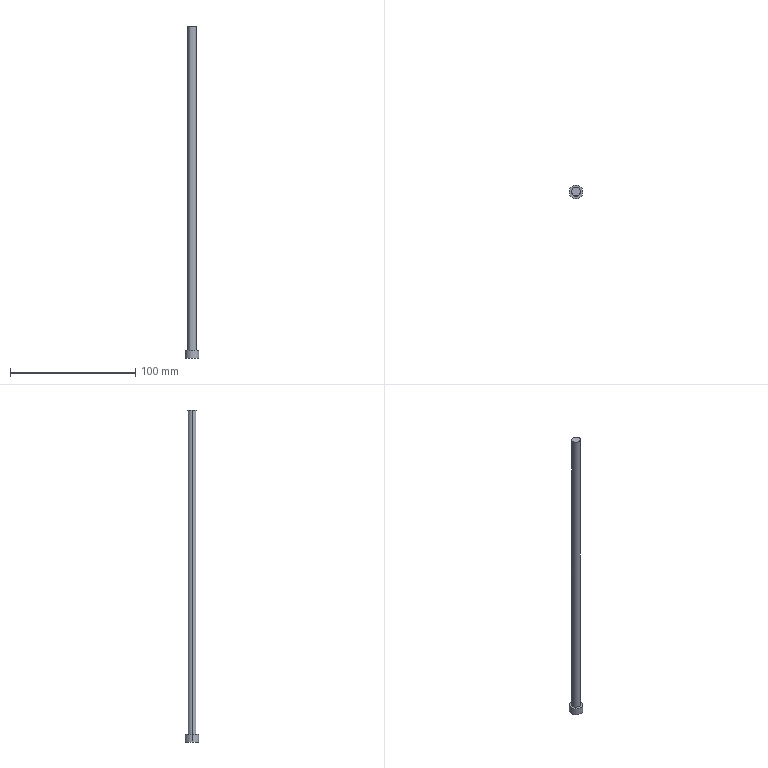Part | Creo | 1 solid | 7 faces | box 11 x 11 x 265.581 mm | volume 10560 mm3 | cylinder 4 | plane 3 | commonest cylinder face diameters 7 x2 11 x2
STEP:
#1=CARTESIAN_POINT('',(0.,0.,0.));
#2=DIRECTION('',(0.,0.,1.));
#3=DIRECTION('',(1.,0.,0.));
#4=AXIS2_PLACEMENT_3D('',#1,#2,#3);
#5=CARTESIAN_POINT('',(3.5,-45.2,-219.5));
#6=VERTEX_POINT('',#5);
#7=CARTESIAN_POINT('',(10.5,-45.2,-219.5));
#8=VERTEX_POINT('',#7);
#9=CARTESIAN_POINT('',(7.,-45.2,-219.5));
#10=DIRECTION('',(0.,0.,-1.));
#11=DIRECTION('',(-1.,0.,0.));
#12=AXIS2_PLACEMENT_3D('',#9,#10,#11);
#13=CIRCLE('',#12,3.5);
#14=EDGE_CURVE('',#6,#8,#13,.T.);
#15=ORIENTED_EDGE('',*,*,#14,.T.);
#16=CARTESIAN_POINT('',(10.5,-45.2,40.081));
#17=VERTEX_POINT('',#16);
#18=CARTESIAN_POINT('',(10.5,-45.2,40.081));
#19=DIRECTION('',(0.,0.,-1.));
#20=VECTOR('',#19,259.581);
#21=LINE('',#18,#20);
#22=EDGE_CURVE('',#17,#8,#21,.T.);
#23=ORIENTED_EDGE('',*,*,#22,.F.);
#24=CARTESIAN_POINT('',(3.5,-45.2,40.081));
#25=VERTEX_POINT('',#24);
#26=CARTESIAN_POINT('',(7.,-45.2,40.081));
#27=DIRECTION('',(0.,0.,1.));
#28=DIRECTION('',(1.,0.,0.));
#29=AXIS2_PLACEMENT_3D('',#26,#27,#28);
#30=CIRCLE('',#29,3.5);
#31=EDGE_CURVE('',#17,#25,#30,.T.);
#32=ORIENTED_EDGE('',*,*,#31,.T.);
#33=CARTESIAN_POINT('',(3.5,-45.2,40.081));
#34=DIRECTION('',(0.,0.,-1.));
#35=VECTOR('',#34,259.581);
#36=LINE('',#33,#35);
#37=EDGE_CURVE('',#25,#6,#36,.T.);
#38=ORIENTED_EDGE('',*,*,#37,.T.);
#39=EDGE_LOOP('',(#15,#23,#32,#38));
#40=FACE_OUTER_BOUND('',#39,.F.);
#41=CARTESIAN_POINT('',(7.,-45.2,125.91));
#42=DIRECTION('',(0.,0.,-1.));
#43=DIRECTION('',(-1.,0.,0.));
#44=AXIS2_PLACEMENT_3D('',#41,#42,#43);
#45=CYLINDRICAL_SURFACE('',#44,3.5);
#46=ADVANCED_FACE('',(#40),#45,.T.);
#47=CARTESIAN_POINT('',(1.5,-45.2,-219.5));
#48=VERTEX_POINT('',#47);
#49=CARTESIAN_POINT('',(12.5,-45.2,-219.5));
#50=VERTEX_POINT('',#49);
#51=CARTESIAN_POINT('',(7.,-45.2,-219.5));
#52=DIRECTION('',(0.,0.,1.));
#53=DIRECTION('',(-1.,0.,0.));
#54=AXIS2_PLACEMENT_3D('',#51,#52,#53);
#55=CIRCLE('',#54,5.5);
#56=EDGE_CURVE('',#48,#50,#55,.T.);
#57=ORIENTED_EDGE('',*,*,#56,.F.);
#58=CARTESIAN_POINT('',(7.,-45.2,-219.5));
#59=DIRECTION('',(0.,0.,1.));
#60=DIRECTION('',(1.,0.,0.));
#61=AXIS2_PLACEMENT_3D('',#58,#59,#60);
#62=CIRCLE('',#61,5.5);
#63=EDGE_CURVE('',#50,#48,#62,.T.);
#64=ORIENTED_EDGE('',*,*,#63,.F.);
#65=EDGE_LOOP('',(#57,#64));
#66=FACE_OUTER_BOUND('',#65,.F.);
#67=ORIENTED_EDGE('',*,*,#14,.F.);
#68=CARTESIAN_POINT('',(7.,-45.2,-219.5));
#69=DIRECTION('',(0.,0.,-1.));
#70=DIRECTION('',(1.,0.,0.));
#71=AXIS2_PLACEMENT_3D('',#68,#69,#70);
#72=CIRCLE('',#71,3.5);
#73=EDGE_CURVE('',#8,#6,#72,.T.);
#74=ORIENTED_EDGE('',*,*,#73,.F.);
#75=EDGE_LOOP('',(#67,#74));
#76=FACE_BOUND('',#75,.F.);
#77=CARTESIAN_POINT('',(-30.,-4.2,-219.5));
#78=DIRECTION('',(0.,0.,-1.));
#79=DIRECTION('',(-1.,0.,0.));
#80=AXIS2_PLACEMENT_3D('',#77,#78,#79);
#81=PLANE('',#80);
#82=ADVANCED_FACE('',(#66,#76),#81,.F.);
#83=CARTESIAN_POINT('',(12.5,-45.2,-225.5));
#84=VERTEX_POINT('',#83);
#85=CARTESIAN_POINT('',(1.5,-45.2,-225.5));
#86=VERTEX_POINT('',#85);
#87=CARTESIAN_POINT('',(7.,-45.2,-225.5));
#88=DIRECTION('',(0.,0.,-1.));
#89=DIRECTION('',(1.,0.,0.));
#90=AXIS2_PLACEMENT_3D('',#87,#88,#89);
#91=CIRCLE('',#90,5.5);
#92=EDGE_CURVE('',#84,#86,#91,.T.);
#93=ORIENTED_EDGE('',*,*,#92,.T.);
#94=CARTESIAN_POINT('',(1.5,-45.2,-225.5));
#95=DIRECTION('',(0.,0.,1.));
#96=VECTOR('',#95,6.);
#97=LINE('',#94,#96);
#98=EDGE_CURVE('',#86,#48,#97,.T.);
#99=ORIENTED_EDGE('',*,*,#98,.T.);
#100=ORIENTED_EDGE('',*,*,#56,.T.);
#101=CARTESIAN_POINT('',(12.5,-45.2,-225.5));
#102=DIRECTION('',(0.,0.,1.));
#103=VECTOR('',#102,6.);
#104=LINE('',#101,#103);
#105=EDGE_CURVE('',#84,#50,#104,.T.);
#106=ORIENTED_EDGE('',*,*,#105,.F.);
#107=EDGE_LOOP('',(#93,#99,#100,#106));
#108=FACE_OUTER_BOUND('',#107,.F.);
#109=CARTESIAN_POINT('',(7.,-45.2,-225.5));
#110=DIRECTION('',(0.,0.,1.));
#111=DIRECTION('',(1.,0.,0.));
#112=AXIS2_PLACEMENT_3D('',#109,#110,#111);
#113=CYLINDRICAL_SURFACE('',#112,5.5);
#114=ADVANCED_FACE('',(#108),#113,.T.);
#115=CARTESIAN_POINT('',(7.,-45.2,-225.5));
#116=DIRECTION('',(0.,0.,-1.));
#117=DIRECTION('',(-1.,0.,0.));
#118=AXIS2_PLACEMENT_3D('',#115,#116,#117);
#119=CIRCLE('',#118,5.5);
#120=EDGE_CURVE('',#86,#84,#119,.T.);
#121=ORIENTED_EDGE('',*,*,#120,.F.);
#122=ORIENTED_EDGE('',*,*,#92,.F.);
#123=EDGE_LOOP('',(#121,#122));
#124=FACE_OUTER_BOUND('',#123,.F.);
#125=CARTESIAN_POINT('',(-30.,-4.2,-225.5));
#126=DIRECTION('',(0.,0.,-1.));
#127=DIRECTION('',(-1.,0.,0.));
#128=AXIS2_PLACEMENT_3D('',#125,#126,#127);
#129=PLANE('',#128);
#130=ADVANCED_FACE('',(#124),#129,.T.);
#131=ORIENTED_EDGE('',*,*,#120,.T.);
#132=ORIENTED_EDGE('',*,*,#105,.T.);
#133=ORIENTED_EDGE('',*,*,#63,.T.);
#134=ORIENTED_EDGE('',*,*,#98,.F.);
#135=EDGE_LOOP('',(#131,#132,#133,#134));
#136=FACE_OUTER_BOUND('',#135,.F.);
#137=CARTESIAN_POINT('',(7.,-45.2,-225.5));
#138=DIRECTION('',(0.,0.,1.));
#139=DIRECTION('',(1.,0.,0.));
#140=AXIS2_PLACEMENT_3D('',#137,#138,#139);
#141=CYLINDRICAL_SURFACE('',#140,5.5);
#142=ADVANCED_FACE('',(#136),#141,.T.);
#143=ORIENTED_EDGE('',*,*,#73,.T.);
#144=ORIENTED_EDGE('',*,*,#37,.F.);
#145=CARTESIAN_POINT('',(7.,-45.2,40.081));
#146=DIRECTION('',(0.,0.,1.));
#147=DIRECTION('',(-1.,0.,0.));
#148=AXIS2_PLACEMENT_3D('',#145,#146,#147);
#149=CIRCLE('',#148,3.5);
#150=EDGE_CURVE('',#25,#17,#149,.T.);
#151=ORIENTED_EDGE('',*,*,#150,.T.);
#152=ORIENTED_EDGE('',*,*,#22,.T.);
#153=EDGE_LOOP('',(#143,#144,#151,#152));
#154=FACE_OUTER_BOUND('',#153,.F.);
#155=CARTESIAN_POINT('',(7.,-45.2,125.91));
#156=DIRECTION('',(0.,0.,-1.));
#157=DIRECTION('',(-1.,0.,0.));
#158=AXIS2_PLACEMENT_3D('',#155,#156,#157);
#159=CYLINDRICAL_SURFACE('',#158,3.5);
#160=ADVANCED_FACE('',(#154),#159,.T.);
#161=ORIENTED_EDGE('',*,*,#31,.F.);
#162=ORIENTED_EDGE('',*,*,#150,.F.);
#163=EDGE_LOOP('',(#161,#162));
#164=FACE_OUTER_BOUND('',#163,.F.);
#165=CARTESIAN_POINT('',(-11.653,-0.6637,40.081));
#166=DIRECTION('',(0.,0.,1.));
#167=DIRECTION('',(1.,0.,0.));
#168=AXIS2_PLACEMENT_3D('',#165,#166,#167);
#169=PLANE('',#168);
#170=ADVANCED_FACE('',(#164),#169,.T.);
#171=CLOSED_SHELL('',(#46,#82,#114,#130,#142,#160,#170));
#172=MANIFOLD_SOLID_BREP('',#171);
#173=(LENGTH_UNIT()NAMED_UNIT(*)SI_UNIT(.MILLI.,.METRE.));
#174=UNCERTAINTY_MEASURE_WITH_UNIT(LENGTH_MEASURE(0.0266),#173,'','');
#175=(NAMED_UNIT(*)PLANE_ANGLE_UNIT()SI_UNIT($,.RADIAN.));
#176=PLANE_ANGLE_MEASURE_WITH_UNIT(PLANE_ANGLE_MEASURE(0.01745),#175);
#177=(CONVERSION_BASED_UNIT('DEGREE',#176)NAMED_UNIT(*)PLANE_ANGLE_UNIT());
#178=(NAMED_UNIT(*)SI_UNIT($,.STERADIAN.)SOLID_ANGLE_UNIT());
#179=(GEOMETRIC_REPRESENTATION_CONTEXT(3)GLOBAL_UNCERTAINTY_ASSIGNED_CONTEXT((#174))GLOBAL_UNIT_ASSIGNED_CONTEXT((#173,#177,#178))REPRESENTATION_CONTEXT('',''));
#180=ADVANCED_BREP_SHAPE_REPRESENTATION('',(#4,#172),#179);